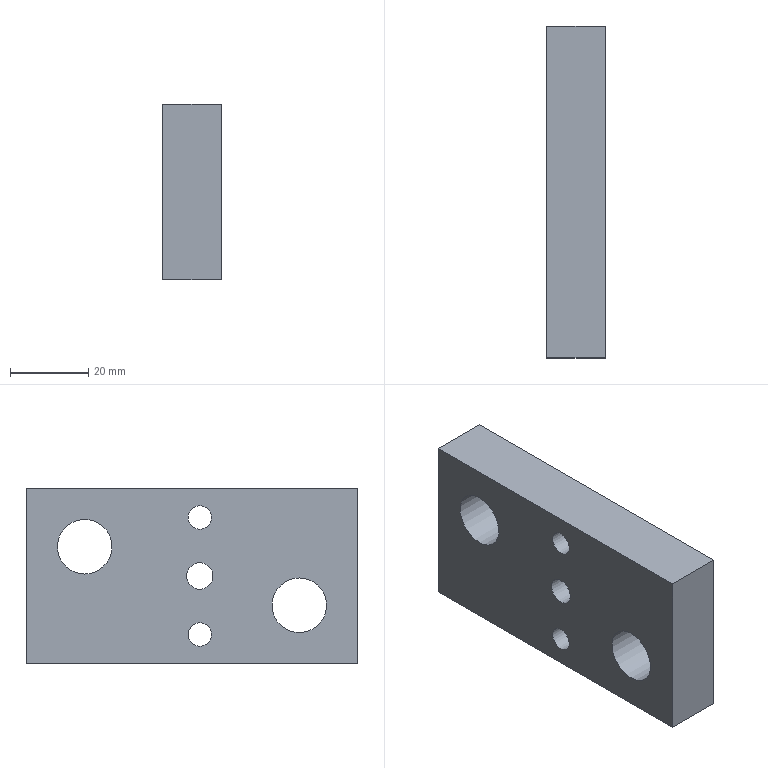Part | NX | features BREP 1 | 1 solid | 15 faces | box 15 x 85 x 45 mm | volume 50757 mm3 | cylinder 7 | plane 6 | cone 2 | commonest cylinder face diameters 5 x2 6 x2 14 x2 6.8 x1
STEP:
#1=CARTESIAN_POINT('',(-2.5,3.,-22.5));
#2=VERTEX_POINT('',#1);
#3=CARTESIAN_POINT('',(0.,3.,-22.5));
#4=DIRECTION('',(0.,0.,-1.));
#5=DIRECTION('',(-1.,0.,0.));
#6=AXIS2_PLACEMENT_3D('',#3,#4,#5);
#7=CIRCLE('',#6,2.5);
#8=EDGE_CURVE('',#2,#2,#7,.T.);
#9=ORIENTED_EDGE('',*,*,#8,.F.);
#10=EDGE_LOOP('',(#9));
#11=FACE_BOUND('',#10,.T.);
#12=CARTESIAN_POINT('',(-7.5,-42.5,-22.5));
#13=VERTEX_POINT('',#12);
#14=CARTESIAN_POINT('',(-7.5,42.5,-22.5));
#15=VERTEX_POINT('',#14);
#16=CARTESIAN_POINT('',(-7.5,-42.5,-22.5));
#17=DIRECTION('',(0.,1.,0.));
#18=VECTOR('',#17,1000.);
#19=LINE('',#16,#18);
#20=EDGE_CURVE('',#13,#15,#19,.T.);
#21=ORIENTED_EDGE('',*,*,#20,.T.);
#22=CARTESIAN_POINT('',(7.5,42.5,-22.5));
#23=VERTEX_POINT('',#22);
#24=CARTESIAN_POINT('',(7.5,42.5,-22.5));
#25=DIRECTION('',(-1.,0.,0.));
#26=VECTOR('',#25,1000.);
#27=LINE('',#24,#26);
#28=EDGE_CURVE('',#23,#15,#27,.T.);
#29=ORIENTED_EDGE('',*,*,#28,.F.);
#30=CARTESIAN_POINT('',(7.5,-42.5,-22.5));
#31=VERTEX_POINT('',#30);
#32=CARTESIAN_POINT('',(7.5,-42.5,-22.5));
#33=DIRECTION('',(0.,1.,0.));
#34=VECTOR('',#33,1000.);
#35=LINE('',#32,#34);
#36=EDGE_CURVE('',#31,#23,#35,.T.);
#37=ORIENTED_EDGE('',*,*,#36,.F.);
#38=CARTESIAN_POINT('',(7.5,-42.5,-22.5));
#39=DIRECTION('',(-1.,0.,0.));
#40=VECTOR('',#39,1000.);
#41=LINE('',#38,#40);
#42=EDGE_CURVE('',#31,#13,#41,.T.);
#43=ORIENTED_EDGE('',*,*,#42,.T.);
#44=EDGE_LOOP('',(#21,#29,#37,#43));
#45=FACE_BOUND('',#44,.T.);
#46=CARTESIAN_POINT('',(7.5,-42.5,-22.5));
#47=DIRECTION('',(0.,0.,1.));
#48=DIRECTION('',(-1.,0.,0.));
#49=AXIS2_PLACEMENT_3D('',#46,#47,#48);
#50=PLANE('',#49);
#51=ADVANCED_FACE('',(#11,#45),#50,.F.);
#52=CARTESIAN_POINT('',(0.,42.5,-1.5));
#53=VERTEX_POINT('',#52);
#54=CARTESIAN_POINT('',(0.,42.5,-4.));
#55=DIRECTION('',(0.,1.,0.));
#56=DIRECTION('',(0.,0.,1.));
#57=AXIS2_PLACEMENT_3D('',#54,#55,#56);
#58=CIRCLE('',#57,2.5);
#59=EDGE_CURVE('',#53,#53,#58,.T.);
#60=ORIENTED_EDGE('',*,*,#59,.F.);
#61=EDGE_LOOP('',(#60));
#62=FACE_BOUND('',#61,.T.);
#63=CARTESIAN_POINT('',(-7.5,42.5,22.5));
#64=VERTEX_POINT('',#63);
#65=CARTESIAN_POINT('',(-7.5,42.5,22.5));
#66=DIRECTION('',(0.,0.,1.));
#67=VECTOR('',#66,1000.);
#68=LINE('',#65,#67);
#69=EDGE_CURVE('',#15,#64,#68,.T.);
#70=ORIENTED_EDGE('',*,*,#69,.T.);
#71=CARTESIAN_POINT('',(7.5,42.5,22.5));
#72=VERTEX_POINT('',#71);
#73=CARTESIAN_POINT('',(7.5,42.5,22.5));
#74=DIRECTION('',(-1.,0.,0.));
#75=VECTOR('',#74,1000.);
#76=LINE('',#73,#75);
#77=EDGE_CURVE('',#72,#64,#76,.T.);
#78=ORIENTED_EDGE('',*,*,#77,.F.);
#79=CARTESIAN_POINT('',(7.5,42.5,22.5));
#80=DIRECTION('',(0.,0.,1.));
#81=VECTOR('',#80,1000.);
#82=LINE('',#79,#81);
#83=EDGE_CURVE('',#23,#72,#82,.T.);
#84=ORIENTED_EDGE('',*,*,#83,.F.);
#85=ORIENTED_EDGE('',*,*,#28,.T.);
#86=EDGE_LOOP('',(#70,#78,#84,#85));
#87=FACE_BOUND('',#86,.T.);
#88=CARTESIAN_POINT('',(7.5,42.5,22.5));
#89=DIRECTION('',(0.,-1.,0.));
#90=DIRECTION('',(0.,0.,1.));
#91=AXIS2_PLACEMENT_3D('',#88,#89,#90);
#92=PLANE('',#91);
#93=ADVANCED_FACE('',(#62,#87),#92,.F.);
#94=CARTESIAN_POINT('',(-7.5,-42.5,22.5));
#95=VERTEX_POINT('',#94);
#96=CARTESIAN_POINT('',(-7.5,-42.5,22.5));
#97=DIRECTION('',(0.,-1.,0.));
#98=VECTOR('',#97,1000.);
#99=LINE('',#96,#98);
#100=EDGE_CURVE('',#64,#95,#99,.T.);
#101=ORIENTED_EDGE('',*,*,#100,.T.);
#102=CARTESIAN_POINT('',(7.5,-42.5,22.5));
#103=VERTEX_POINT('',#102);
#104=CARTESIAN_POINT('',(7.5,-42.5,22.5));
#105=DIRECTION('',(-1.,0.,0.));
#106=VECTOR('',#105,1000.);
#107=LINE('',#104,#106);
#108=EDGE_CURVE('',#103,#95,#107,.T.);
#109=ORIENTED_EDGE('',*,*,#108,.F.);
#110=CARTESIAN_POINT('',(7.5,-42.5,22.5));
#111=DIRECTION('',(0.,-1.,0.));
#112=VECTOR('',#111,1000.);
#113=LINE('',#110,#112);
#114=EDGE_CURVE('',#72,#103,#113,.T.);
#115=ORIENTED_EDGE('',*,*,#114,.F.);
#116=ORIENTED_EDGE('',*,*,#77,.T.);
#117=EDGE_LOOP('',(#101,#109,#115,#116));
#118=FACE_BOUND('',#117,.T.);
#119=CARTESIAN_POINT('',(7.5,-42.5,22.5));
#120=DIRECTION('',(0.,0.,-1.));
#121=DIRECTION('',(1.,0.,0.));
#122=AXIS2_PLACEMENT_3D('',#119,#120,#121);
#123=PLANE('',#122);
#124=ADVANCED_FACE('',(#118),#123,.F.);
#125=CARTESIAN_POINT('',(-7.5,-42.5,22.5));
#126=DIRECTION('',(0.,0.,-1.));
#127=VECTOR('',#126,1000.);
#128=LINE('',#125,#127);
#129=EDGE_CURVE('',#95,#13,#128,.T.);
#130=ORIENTED_EDGE('',*,*,#129,.T.);
#131=ORIENTED_EDGE('',*,*,#42,.F.);
#132=CARTESIAN_POINT('',(7.5,-42.5,22.5));
#133=DIRECTION('',(0.,0.,-1.));
#134=VECTOR('',#133,1000.);
#135=LINE('',#132,#134);
#136=EDGE_CURVE('',#103,#31,#135,.T.);
#137=ORIENTED_EDGE('',*,*,#136,.F.);
#138=ORIENTED_EDGE('',*,*,#108,.T.);
#139=EDGE_LOOP('',(#130,#131,#137,#138));
#140=FACE_BOUND('',#139,.T.);
#141=CARTESIAN_POINT('',(7.5,-42.5,22.5));
#142=DIRECTION('',(0.,1.,0.));
#143=DIRECTION('',(0.,0.,-1.));
#144=AXIS2_PLACEMENT_3D('',#141,#142,#143);
#145=PLANE('',#144);
#146=ADVANCED_FACE('',(#140),#145,.F.);
#147=CARTESIAN_POINT('',(7.5,27.5,14.5));
#148=VERTEX_POINT('',#147);
#149=CARTESIAN_POINT('',(7.5,27.5,7.5));
#150=DIRECTION('',(-1.,0.,0.));
#151=DIRECTION('',(0.,0.,1.));
#152=AXIS2_PLACEMENT_3D('',#149,#150,#151);
#153=CIRCLE('',#152,7.);
#154=EDGE_CURVE('',#148,#148,#153,.T.);
#155=ORIENTED_EDGE('',*,*,#154,.T.);
#156=EDGE_LOOP('',(#155));
#157=FACE_BOUND('',#156,.T.);
#158=CARTESIAN_POINT('',(7.5,-27.5,-0.5));
#159=VERTEX_POINT('',#158);
#160=CARTESIAN_POINT('',(7.5,-27.5,-7.5));
#161=DIRECTION('',(-1.,0.,0.));
#162=DIRECTION('',(0.,0.,1.));
#163=AXIS2_PLACEMENT_3D('',#160,#161,#162);
#164=CIRCLE('',#163,7.);
#165=EDGE_CURVE('',#159,#159,#164,.T.);
#166=ORIENTED_EDGE('',*,*,#165,.T.);
#167=EDGE_LOOP('',(#166));
#168=FACE_BOUND('',#167,.T.);
#169=CARTESIAN_POINT('',(7.5,-2.,-3.4));
#170=VERTEX_POINT('',#169);
#171=CARTESIAN_POINT('',(7.5,-2.,0.));
#172=DIRECTION('',(1.,0.,0.));
#173=DIRECTION('',(0.,0.,-1.));
#174=AXIS2_PLACEMENT_3D('',#171,#172,#173);
#175=CIRCLE('',#174,3.4);
#176=EDGE_CURVE('',#170,#170,#175,.T.);
#177=ORIENTED_EDGE('',*,*,#176,.F.);
#178=EDGE_LOOP('',(#177));
#179=FACE_BOUND('',#178,.T.);
#180=CARTESIAN_POINT('',(7.5,-2.,12.));
#181=VERTEX_POINT('',#180);
#182=CARTESIAN_POINT('',(7.5,-2.,15.));
#183=DIRECTION('',(1.,0.,0.));
#184=DIRECTION('',(0.,0.,-1.));
#185=AXIS2_PLACEMENT_3D('',#182,#183,#184);
#186=CIRCLE('',#185,3.);
#187=EDGE_CURVE('',#181,#181,#186,.T.);
#188=ORIENTED_EDGE('',*,*,#187,.F.);
#189=EDGE_LOOP('',(#188));
#190=FACE_BOUND('',#189,.T.);
#191=CARTESIAN_POINT('',(7.5,-2.,-18.));
#192=VERTEX_POINT('',#191);
#193=CARTESIAN_POINT('',(7.5,-2.,-15.));
#194=DIRECTION('',(1.,0.,0.));
#195=DIRECTION('',(0.,0.,-1.));
#196=AXIS2_PLACEMENT_3D('',#193,#194,#195);
#197=CIRCLE('',#196,3.);
#198=EDGE_CURVE('',#192,#192,#197,.T.);
#199=ORIENTED_EDGE('',*,*,#198,.F.);
#200=EDGE_LOOP('',(#199));
#201=FACE_BOUND('',#200,.T.);
#202=ORIENTED_EDGE('',*,*,#36,.T.);
#203=ORIENTED_EDGE('',*,*,#83,.T.);
#204=ORIENTED_EDGE('',*,*,#114,.T.);
#205=ORIENTED_EDGE('',*,*,#136,.T.);
#206=EDGE_LOOP('',(#202,#203,#204,#205));
#207=FACE_BOUND('',#206,.T.);
#208=CARTESIAN_POINT('',(7.5,0.,0.));
#209=DIRECTION('',(-1.,0.,0.));
#210=DIRECTION('',(0.,0.,-1.));
#211=AXIS2_PLACEMENT_3D('',#208,#209,#210);
#212=PLANE('',#211);
#213=ADVANCED_FACE('',(#157,#168,#179,#190,#201,#207),#212,.F.);
#214=CARTESIAN_POINT('',(-7.5,27.5,14.5));
#215=VERTEX_POINT('',#214);
#216=CARTESIAN_POINT('',(-7.5,27.5,7.5));
#217=DIRECTION('',(-1.,0.,0.));
#218=DIRECTION('',(0.,0.,1.));
#219=AXIS2_PLACEMENT_3D('',#216,#217,#218);
#220=CIRCLE('',#219,7.);
#221=EDGE_CURVE('',#215,#215,#220,.T.);
#222=ORIENTED_EDGE('',*,*,#221,.F.);
#223=EDGE_LOOP('',(#222));
#224=FACE_BOUND('',#223,.T.);
#225=CARTESIAN_POINT('',(-7.5,-27.5,-0.5));
#226=VERTEX_POINT('',#225);
#227=CARTESIAN_POINT('',(-7.5,-27.5,-7.5));
#228=DIRECTION('',(-1.,0.,0.));
#229=DIRECTION('',(0.,0.,1.));
#230=AXIS2_PLACEMENT_3D('',#227,#228,#229);
#231=CIRCLE('',#230,7.);
#232=EDGE_CURVE('',#226,#226,#231,.T.);
#233=ORIENTED_EDGE('',*,*,#232,.F.);
#234=EDGE_LOOP('',(#233));
#235=FACE_BOUND('',#234,.T.);
#236=CARTESIAN_POINT('',(-7.5,-2.,-3.4));
#237=VERTEX_POINT('',#236);
#238=CARTESIAN_POINT('',(-7.5,-2.,0.));
#239=DIRECTION('',(1.,0.,0.));
#240=DIRECTION('',(0.,0.,-1.));
#241=AXIS2_PLACEMENT_3D('',#238,#239,#240);
#242=CIRCLE('',#241,3.4);
#243=EDGE_CURVE('',#237,#237,#242,.T.);
#244=ORIENTED_EDGE('',*,*,#243,.T.);
#245=EDGE_LOOP('',(#244));
#246=FACE_BOUND('',#245,.T.);
#247=CARTESIAN_POINT('',(-7.5,-2.,12.));
#248=VERTEX_POINT('',#247);
#249=CARTESIAN_POINT('',(-7.5,-2.,15.));
#250=DIRECTION('',(1.,0.,0.));
#251=DIRECTION('',(0.,0.,-1.));
#252=AXIS2_PLACEMENT_3D('',#249,#250,#251);
#253=CIRCLE('',#252,3.);
#254=EDGE_CURVE('',#248,#248,#253,.T.);
#255=ORIENTED_EDGE('',*,*,#254,.T.);
#256=EDGE_LOOP('',(#255));
#257=FACE_BOUND('',#256,.T.);
#258=CARTESIAN_POINT('',(-7.5,-2.,-18.));
#259=VERTEX_POINT('',#258);
#260=CARTESIAN_POINT('',(-7.5,-2.,-15.));
#261=DIRECTION('',(1.,0.,0.));
#262=DIRECTION('',(0.,0.,-1.));
#263=AXIS2_PLACEMENT_3D('',#260,#261,#262);
#264=CIRCLE('',#263,3.);
#265=EDGE_CURVE('',#259,#259,#264,.T.);
#266=ORIENTED_EDGE('',*,*,#265,.T.);
#267=EDGE_LOOP('',(#266));
#268=FACE_BOUND('',#267,.T.);
#269=ORIENTED_EDGE('',*,*,#20,.F.);
#270=ORIENTED_EDGE('',*,*,#129,.F.);
#271=ORIENTED_EDGE('',*,*,#100,.F.);
#272=ORIENTED_EDGE('',*,*,#69,.F.);
#273=EDGE_LOOP('',(#269,#270,#271,#272));
#274=FACE_BOUND('',#273,.T.);
#275=CARTESIAN_POINT('',(-7.5,0.,0.));
#276=DIRECTION('',(-1.,0.,0.));
#277=DIRECTION('',(0.,0.,-1.));
#278=AXIS2_PLACEMENT_3D('',#275,#276,#277);
#279=PLANE('',#278);
#280=ADVANCED_FACE('',(#224,#235,#246,#257,#268,#274),#279,.T.);
#281=CARTESIAN_POINT('',(-1.5,1.,-15.));
#282=VERTEX_POINT('',#281);
#283=CARTESIAN_POINT('',(-1.266,0.7727,-16.3));
#284=CARTESIAN_POINT('',(-1.617,1.113,-14.999));
#285=CARTESIAN_POINT('',(-1.266,0.774,-13.704));
#286=CARTESIAN_POINT('',(-0.00499,0.3634,-13.162));
#287=CARTESIAN_POINT('',(1.265,0.7724,-13.7));
#288=CARTESIAN_POINT('',(1.617,1.113,-15.));
#289=CARTESIAN_POINT('',(1.267,0.7749,-16.295));
#290=CARTESIAN_POINT('',(0.005814,0.3631,-16.839));
#291=CARTESIAN_POINT('',(-1.266,0.7727,-16.3));
#292=CARTESIAN_POINT('',(-1.617,1.113,-14.999));
#293=CARTESIAN_POINT('',(-1.266,0.774,-13.704));
#294=B_SPLINE_CURVE_WITH_KNOTS('',3,(#283,#284,#285,#286,#287,#288,#289,#290,#291,#292,#293),.UNSPECIFIED.,.T.,.F.,(1,1,1,1,1,1,1,1,1,1,1,1,1,1,1),(-0.003843,-0.002562,-0.001281,0.,0.001281,0.002562,0.003843,0.005123,0.006404,0.007685,0.008966,0.01025,0.01153,0.01281,0.01409),.UNSPECIFIED.);
#295=EDGE_CURVE('',#282,#282,#294,.T.);
#296=ORIENTED_EDGE('',*,*,#295,.T.);
#297=EDGE_LOOP('',(#296));
#298=FACE_BOUND('',#297,.T.);
#299=ORIENTED_EDGE('',*,*,#265,.F.);
#300=EDGE_LOOP('',(#299));
#301=FACE_BOUND('',#300,.T.);
#302=ORIENTED_EDGE('',*,*,#198,.T.);
#303=EDGE_LOOP('',(#302));
#304=FACE_BOUND('',#303,.T.);
#305=CARTESIAN_POINT('',(7.5,-2.,-15.));
#306=DIRECTION('',(1.,0.,0.));
#307=DIRECTION('',(0.,0.,1.));
#308=AXIS2_PLACEMENT_3D('',#305,#306,#307);
#309=CYLINDRICAL_SURFACE('',#308,3.);
#310=ADVANCED_FACE('',(#298,#301,#304),#309,.F.);
#311=ORIENTED_EDGE('',*,*,#254,.F.);
#312=EDGE_LOOP('',(#311));
#313=FACE_BOUND('',#312,.T.);
#314=ORIENTED_EDGE('',*,*,#187,.T.);
#315=EDGE_LOOP('',(#314));
#316=FACE_BOUND('',#315,.T.);
#317=CARTESIAN_POINT('',(7.5,-2.,15.));
#318=DIRECTION('',(1.,0.,0.));
#319=DIRECTION('',(0.,0.,1.));
#320=AXIS2_PLACEMENT_3D('',#317,#318,#319);
#321=CYLINDRICAL_SURFACE('',#320,3.);
#322=ADVANCED_FACE('',(#313,#316),#321,.F.);
#323=ORIENTED_EDGE('',*,*,#243,.F.);
#324=EDGE_LOOP('',(#323));
#325=FACE_BOUND('',#324,.T.);
#326=ORIENTED_EDGE('',*,*,#176,.T.);
#327=EDGE_LOOP('',(#326));
#328=FACE_BOUND('',#327,.T.);
#329=CARTESIAN_POINT('',(7.5,-2.,0.));
#330=DIRECTION('',(1.,0.,0.));
#331=DIRECTION('',(0.,0.,1.));
#332=AXIS2_PLACEMENT_3D('',#329,#330,#331);
#333=CYLINDRICAL_SURFACE('',#332,3.4);
#334=ADVANCED_FACE('',(#325,#328),#333,.F.);
#335=ORIENTED_EDGE('',*,*,#8,.T.);
#336=EDGE_LOOP('',(#335));
#337=FACE_BOUND('',#336,.T.);
#338=CARTESIAN_POINT('',(-2.5,3.,-7.5));
#339=VERTEX_POINT('',#338);
#340=CARTESIAN_POINT('',(0.,3.,-7.5));
#341=DIRECTION('',(0.,0.,-1.));
#342=DIRECTION('',(-1.,0.,0.));
#343=AXIS2_PLACEMENT_3D('',#340,#341,#342);
#344=CIRCLE('',#343,2.5);
#345=EDGE_CURVE('',#339,#339,#344,.T.);
#346=ORIENTED_EDGE('',*,*,#345,.F.);
#347=EDGE_LOOP('',(#346));
#348=FACE_BOUND('',#347,.T.);
#349=ORIENTED_EDGE('',*,*,#295,.F.);
#350=EDGE_LOOP('',(#349));
#351=FACE_BOUND('',#350,.T.);
#352=CARTESIAN_POINT('',(0.,3.,-22.5));
#353=DIRECTION('',(0.,0.,-1.));
#354=DIRECTION('',(1.,0.,0.));
#355=AXIS2_PLACEMENT_3D('',#352,#353,#354);
#356=CYLINDRICAL_SURFACE('',#355,2.5);
#357=ADVANCED_FACE('',(#337,#348,#351),#356,.F.);
#358=CARTESIAN_POINT('',(0.,3.,-5.998));
#359=VERTEX_POINT('',#358);
#360=VERTEX_LOOP('',#359);
#361=FACE_BOUND('',#360,.T.);
#362=ORIENTED_EDGE('',*,*,#345,.T.);
#363=EDGE_LOOP('',(#362));
#364=FACE_BOUND('',#363,.T.);
#365=CARTESIAN_POINT('',(0.,3.,-7.5));
#366=DIRECTION('',(0.,0.,-1.));
#367=DIRECTION('',(1.,0.,0.));
#368=AXIS2_PLACEMENT_3D('',#365,#366,#367);
#369=CONICAL_SURFACE('',#368,2.5,1.03);
#370=ADVANCED_FACE('',(#361,#364),#369,.F.);
#371=CARTESIAN_POINT('',(0.,25.998,-4.));
#372=VERTEX_POINT('',#371);
#373=VERTEX_LOOP('',#372);
#374=FACE_BOUND('',#373,.T.);
#375=CARTESIAN_POINT('',(0.,27.5,-1.5));
#376=VERTEX_POINT('',#375);
#377=CARTESIAN_POINT('',(0.,27.5,-4.));
#378=DIRECTION('',(0.,1.,0.));
#379=DIRECTION('',(0.,0.,1.));
#380=AXIS2_PLACEMENT_3D('',#377,#378,#379);
#381=CIRCLE('',#380,2.5);
#382=EDGE_CURVE('',#376,#376,#381,.T.);
#383=ORIENTED_EDGE('',*,*,#382,.T.);
#384=EDGE_LOOP('',(#383));
#385=FACE_BOUND('',#384,.T.);
#386=CARTESIAN_POINT('',(0.,27.5,-4.));
#387=DIRECTION('',(0.,1.,0.));
#388=DIRECTION('',(0.,0.,-1.));
#389=AXIS2_PLACEMENT_3D('',#386,#387,#388);
#390=CONICAL_SURFACE('',#389,2.5,1.03);
#391=ADVANCED_FACE('',(#374,#385),#390,.F.);
#392=ORIENTED_EDGE('',*,*,#382,.F.);
#393=EDGE_LOOP('',(#392));
#394=FACE_BOUND('',#393,.T.);
#395=ORIENTED_EDGE('',*,*,#59,.T.);
#396=EDGE_LOOP('',(#395));
#397=FACE_BOUND('',#396,.T.);
#398=CARTESIAN_POINT('',(0.,42.5,-4.));
#399=DIRECTION('',(0.,1.,0.));
#400=DIRECTION('',(0.,0.,-1.));
#401=AXIS2_PLACEMENT_3D('',#398,#399,#400);
#402=CYLINDRICAL_SURFACE('',#401,2.5);
#403=ADVANCED_FACE('',(#394,#397),#402,.F.);
#404=ORIENTED_EDGE('',*,*,#165,.F.);
#405=EDGE_LOOP('',(#404));
#406=FACE_BOUND('',#405,.T.);
#407=ORIENTED_EDGE('',*,*,#232,.T.);
#408=EDGE_LOOP('',(#407));
#409=FACE_BOUND('',#408,.T.);
#410=CARTESIAN_POINT('',(-7.5,-27.5,-7.5));
#411=DIRECTION('',(-1.,0.,0.));
#412=DIRECTION('',(0.,0.,-1.));
#413=AXIS2_PLACEMENT_3D('',#410,#411,#412);
#414=CYLINDRICAL_SURFACE('',#413,7.);
#415=ADVANCED_FACE('',(#406,#409),#414,.F.);
#416=ORIENTED_EDGE('',*,*,#154,.F.);
#417=EDGE_LOOP('',(#416));
#418=FACE_BOUND('',#417,.T.);
#419=ORIENTED_EDGE('',*,*,#221,.T.);
#420=EDGE_LOOP('',(#419));
#421=FACE_BOUND('',#420,.T.);
#422=CARTESIAN_POINT('',(-7.5,27.5,7.5));
#423=DIRECTION('',(-1.,0.,0.));
#424=DIRECTION('',(0.,0.,-1.));
#425=AXIS2_PLACEMENT_3D('',#422,#423,#424);
#426=CYLINDRICAL_SURFACE('',#425,7.);
#427=ADVANCED_FACE('',(#418,#421),#426,.F.);
#428=CLOSED_SHELL('',(#51,#93,#124,#146,#213,#280,#310,#322,#334,#357,#370,#391,#403,#415,#427));
#429=MANIFOLD_SOLID_BREP('',#428);
#430=(LENGTH_UNIT()NAMED_UNIT(*)SI_UNIT(.MILLI.,.METRE.));
#431=UNCERTAINTY_MEASURE_WITH_UNIT(LENGTH_MEASURE(0.0508),#430,'','');
#432=(NAMED_UNIT(*)PLANE_ANGLE_UNIT()SI_UNIT($,.RADIAN.));
#433=(NAMED_UNIT(*)SI_UNIT($,.STERADIAN.)SOLID_ANGLE_UNIT());
#434=(GEOMETRIC_REPRESENTATION_CONTEXT(3)GLOBAL_UNCERTAINTY_ASSIGNED_CONTEXT((#431))GLOBAL_UNIT_ASSIGNED_CONTEXT((#430,#432,#433))REPRESENTATION_CONTEXT('',''));
#435=ADVANCED_BREP_SHAPE_REPRESENTATION('',(#429),#434);